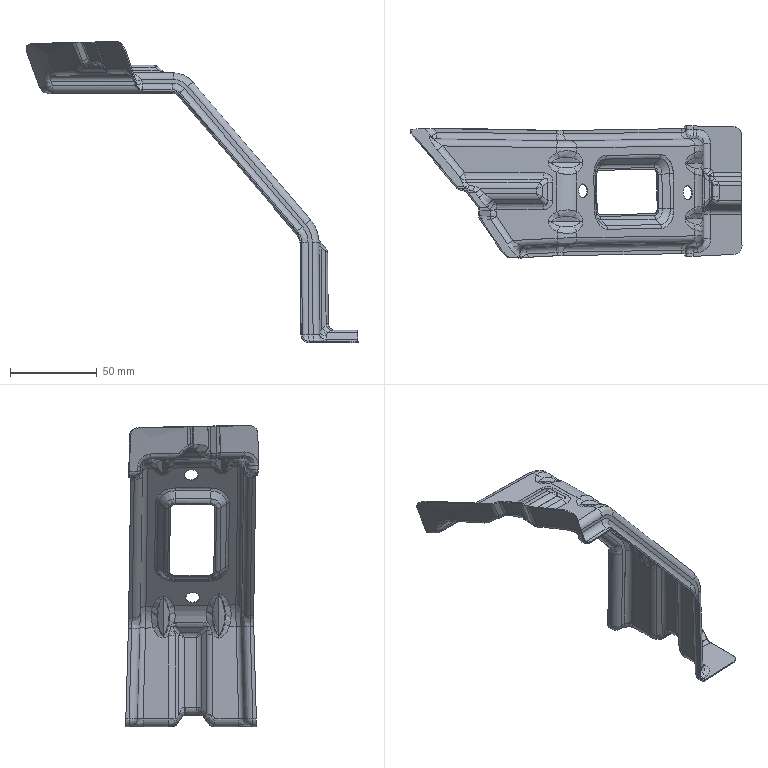Part | 1 solid | 479 faces | box 190.968 x 76.286 x 173.359 mm | volume 15703 mm3 | spline 317 | cylinder 128 | plane 18 | other 9 | sphere 7 | commonest cylinder face diameters 8 x27 6 x20 9.4 x17 10 x13 4.6 x10 8.6 x8